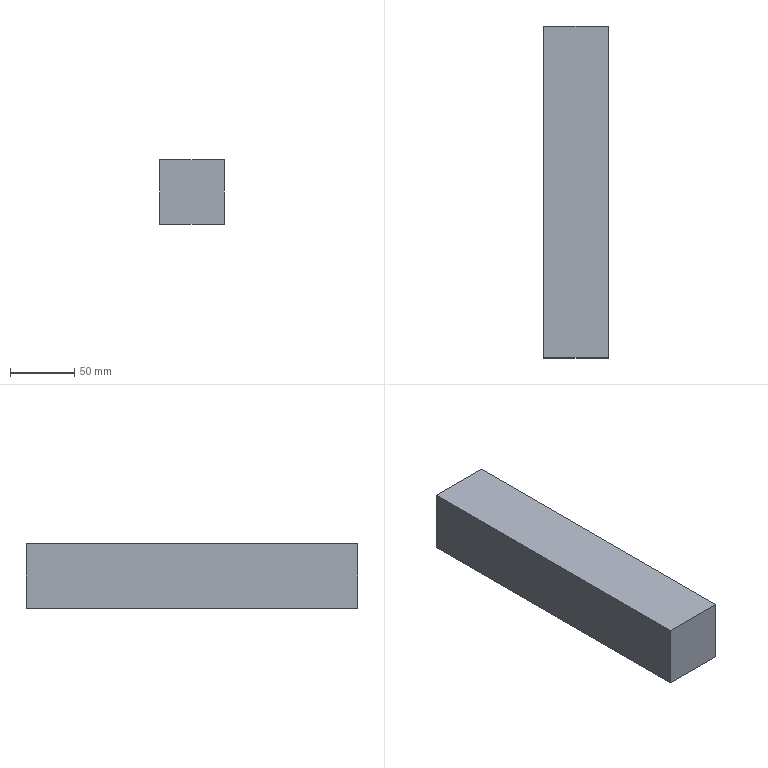Part | STEP file | 1 solid | 6 faces | box 50 x 259.164 x 50 mm | volume 647910 mm3 | plane 6
STEP:
#1=CARTESIAN_POINT('',(0.,0.,0.));
#2=DIRECTION('',(0.,0.,1.));
#3=DIRECTION('',(1.,0.,0.));
#4=AXIS2_PLACEMENT_3D('',#1,#2,#3);
#5=CARTESIAN_POINT('',(294.689,-240.836,393.641));
#6=VERTEX_POINT('',#5);
#7=CARTESIAN_POINT('',(294.689,-500.,393.641));
#8=VERTEX_POINT('',#7);
#9=CARTESIAN_POINT('',(294.689,-240.836,393.641));
#10=DIRECTION('',(0.,-1.,0.));
#11=VECTOR('',#10,1.);
#12=LINE('',#9,#11);
#13=CARTESIAN_POINT('',(294.689,-240.836,343.641));
#14=DIRECTION('',(1.,0.,0.));
#15=DIRECTION('',(0.,0.,1.));
#16=AXIS2_PLACEMENT_3D('',#13,#14,#15);
#17=PLANE('',#16);
#18=CARTESIAN_POINT('',(50.,0.));
#19=DIRECTION('',(0.,1.));
#20=VECTOR('',#19,1.);
#21=LINE('',#18,#20);
#22=(GEOMETRIC_REPRESENTATION_CONTEXT(2)PARAMETRIC_REPRESENTATION_CONTEXT()REPRESENTATION_CONTEXT('',''));
#23=DEFINITIONAL_REPRESENTATION('',(#21),#22);
#24=PCURVE('',#17,#23);
#25=CARTESIAN_POINT('',(0.,0.,393.641));
#26=DIRECTION('',(0.,0.,1.));
#27=DIRECTION('',(-1.,0.,0.));
#28=AXIS2_PLACEMENT_3D('',#25,#26,#27);
#29=PLANE('',#28);
#30=CARTESIAN_POINT('',(-294.689,240.836));
#31=DIRECTION('',(0.,1.));
#32=VECTOR('',#31,1.);
#33=LINE('',#30,#32);
#34=(GEOMETRIC_REPRESENTATION_CONTEXT(2)PARAMETRIC_REPRESENTATION_CONTEXT()REPRESENTATION_CONTEXT('',''));
#35=DEFINITIONAL_REPRESENTATION('',(#33),#34);
#36=PCURVE('',#29,#35);
#37=SURFACE_CURVE('',#12,(#24,#36),.PCURVE_S1.);
#38=EDGE_CURVE('',#6,#8,#37,.T.);
#39=ORIENTED_EDGE('',*,*,#38,.T.);
#40=CARTESIAN_POINT('',(294.689,-500.,343.641));
#41=VERTEX_POINT('',#40);
#42=CARTESIAN_POINT('',(294.689,-500.,343.641));
#43=DIRECTION('',(0.,0.,1.));
#44=VECTOR('',#43,1.);
#45=LINE('',#42,#44);
#46=CARTESIAN_POINT('',(0.,259.164));
#47=DIRECTION('',(1.,0.));
#48=VECTOR('',#47,1.);
#49=LINE('',#46,#48);
#50=(GEOMETRIC_REPRESENTATION_CONTEXT(2)PARAMETRIC_REPRESENTATION_CONTEXT()REPRESENTATION_CONTEXT('',''));
#51=DEFINITIONAL_REPRESENTATION('',(#49),#50);
#52=PCURVE('',#17,#51);
#53=CARTESIAN_POINT('',(294.689,-500.,343.641));
#54=DIRECTION('',(0.,-1.,0.));
#55=DIRECTION('',(-1.,0.,0.));
#56=AXIS2_PLACEMENT_3D('',#53,#54,#55);
#57=PLANE('',#56);
#58=CARTESIAN_POINT('',(0.,0.));
#59=DIRECTION('',(0.,-1.));
#60=VECTOR('',#59,1.);
#61=LINE('',#58,#60);
#62=(GEOMETRIC_REPRESENTATION_CONTEXT(2)PARAMETRIC_REPRESENTATION_CONTEXT()REPRESENTATION_CONTEXT('',''));
#63=DEFINITIONAL_REPRESENTATION('',(#61),#62);
#64=PCURVE('',#57,#63);
#65=SURFACE_CURVE('',#45,(#52,#64),.PCURVE_S1.);
#66=EDGE_CURVE('',#41,#8,#65,.T.);
#67=ORIENTED_EDGE('',*,*,#66,.F.);
#68=CARTESIAN_POINT('',(294.689,-240.836,343.641));
#69=VERTEX_POINT('',#68);
#70=CARTESIAN_POINT('',(294.689,-240.836,343.641));
#71=DIRECTION('',(0.,-1.,0.));
#72=VECTOR('',#71,1.);
#73=LINE('',#70,#72);
#74=CARTESIAN_POINT('',(0.,0.));
#75=DIRECTION('',(0.,1.));
#76=VECTOR('',#75,1.);
#77=LINE('',#74,#76);
#78=(GEOMETRIC_REPRESENTATION_CONTEXT(2)PARAMETRIC_REPRESENTATION_CONTEXT()REPRESENTATION_CONTEXT('',''));
#79=DEFINITIONAL_REPRESENTATION('',(#77),#78);
#80=PCURVE('',#17,#79);
#81=CARTESIAN_POINT('',(0.,0.,343.641));
#82=DIRECTION('',(0.,0.,1.));
#83=DIRECTION('',(-1.,0.,0.));
#84=AXIS2_PLACEMENT_3D('',#81,#82,#83);
#85=PLANE('',#84);
#86=CARTESIAN_POINT('',(-294.689,240.836));
#87=DIRECTION('',(0.,1.));
#88=VECTOR('',#87,1.);
#89=LINE('',#86,#88);
#90=(GEOMETRIC_REPRESENTATION_CONTEXT(2)PARAMETRIC_REPRESENTATION_CONTEXT()REPRESENTATION_CONTEXT('',''));
#91=DEFINITIONAL_REPRESENTATION('',(#89),#90);
#92=PCURVE('',#85,#91);
#93=SURFACE_CURVE('',#73,(#80,#92),.PCURVE_S1.);
#94=EDGE_CURVE('',#69,#41,#93,.T.);
#95=ORIENTED_EDGE('',*,*,#94,.F.);
#96=CARTESIAN_POINT('',(294.689,-240.836,343.641));
#97=DIRECTION('',(0.,0.,1.));
#98=VECTOR('',#97,1.);
#99=LINE('',#96,#98);
#100=CARTESIAN_POINT('',(0.,0.));
#101=DIRECTION('',(1.,0.));
#102=VECTOR('',#101,1.);
#103=LINE('',#100,#102);
#104=(GEOMETRIC_REPRESENTATION_CONTEXT(2)PARAMETRIC_REPRESENTATION_CONTEXT()REPRESENTATION_CONTEXT('',''));
#105=DEFINITIONAL_REPRESENTATION('',(#103),#104);
#106=PCURVE('',#17,#105);
#107=CARTESIAN_POINT('',(294.689,-240.836,343.641));
#108=DIRECTION('',(0.,1.,0.));
#109=DIRECTION('',(1.,0.,0.));
#110=AXIS2_PLACEMENT_3D('',#107,#108,#109);
#111=PLANE('',#110);
#112=CARTESIAN_POINT('',(0.,0.));
#113=DIRECTION('',(0.,-1.));
#114=VECTOR('',#113,1.);
#115=LINE('',#112,#114);
#116=(GEOMETRIC_REPRESENTATION_CONTEXT(2)PARAMETRIC_REPRESENTATION_CONTEXT()REPRESENTATION_CONTEXT('',''));
#117=DEFINITIONAL_REPRESENTATION('',(#115),#116);
#118=PCURVE('',#111,#117);
#119=SURFACE_CURVE('',#99,(#106,#118),.PCURVE_S1.);
#120=EDGE_CURVE('',#69,#6,#119,.T.);
#121=ORIENTED_EDGE('',*,*,#120,.T.);
#122=EDGE_LOOP('',(#39,#67,#95,#121));
#123=FACE_BOUND('',#122,.T.);
#124=ADVANCED_FACE('',(#123),#17,.T.);
#125=CARTESIAN_POINT('',(244.689,-240.836,393.641));
#126=VERTEX_POINT('',#125);
#127=CARTESIAN_POINT('',(294.689,-240.836,393.641));
#128=DIRECTION('',(1.,0.,0.));
#129=VECTOR('',#128,1.);
#130=LINE('',#127,#129);
#131=CARTESIAN_POINT('',(0.,-50.));
#132=DIRECTION('',(1.,0.));
#133=VECTOR('',#132,1.);
#134=LINE('',#131,#133);
#135=(GEOMETRIC_REPRESENTATION_CONTEXT(2)PARAMETRIC_REPRESENTATION_CONTEXT()REPRESENTATION_CONTEXT('',''));
#136=DEFINITIONAL_REPRESENTATION('',(#134),#135);
#137=PCURVE('',#111,#136);
#138=CARTESIAN_POINT('',(-294.689,240.836));
#139=DIRECTION('',(-1.,0.));
#140=VECTOR('',#139,1.);
#141=LINE('',#138,#140);
#142=(GEOMETRIC_REPRESENTATION_CONTEXT(2)PARAMETRIC_REPRESENTATION_CONTEXT()REPRESENTATION_CONTEXT('',''));
#143=DEFINITIONAL_REPRESENTATION('',(#141),#142);
#144=PCURVE('',#29,#143);
#145=SURFACE_CURVE('',#130,(#137,#144),.PCURVE_S1.);
#146=EDGE_CURVE('',#126,#6,#145,.T.);
#147=ORIENTED_EDGE('',*,*,#146,.T.);
#148=ORIENTED_EDGE('',*,*,#120,.F.);
#149=CARTESIAN_POINT('',(244.689,-240.836,343.641));
#150=VERTEX_POINT('',#149);
#151=CARTESIAN_POINT('',(294.689,-240.836,343.641));
#152=DIRECTION('',(1.,0.,0.));
#153=VECTOR('',#152,1.);
#154=LINE('',#151,#153);
#155=CARTESIAN_POINT('',(0.,0.));
#156=DIRECTION('',(1.,0.));
#157=VECTOR('',#156,1.);
#158=LINE('',#155,#157);
#159=(GEOMETRIC_REPRESENTATION_CONTEXT(2)PARAMETRIC_REPRESENTATION_CONTEXT()REPRESENTATION_CONTEXT('',''));
#160=DEFINITIONAL_REPRESENTATION('',(#158),#159);
#161=PCURVE('',#111,#160);
#162=CARTESIAN_POINT('',(-294.689,240.836));
#163=DIRECTION('',(-1.,0.));
#164=VECTOR('',#163,1.);
#165=LINE('',#162,#164);
#166=(GEOMETRIC_REPRESENTATION_CONTEXT(2)PARAMETRIC_REPRESENTATION_CONTEXT()REPRESENTATION_CONTEXT('',''));
#167=DEFINITIONAL_REPRESENTATION('',(#165),#166);
#168=PCURVE('',#85,#167);
#169=SURFACE_CURVE('',#154,(#161,#168),.PCURVE_S1.);
#170=EDGE_CURVE('',#150,#69,#169,.T.);
#171=ORIENTED_EDGE('',*,*,#170,.F.);
#172=CARTESIAN_POINT('',(244.689,-240.836,343.641));
#173=DIRECTION('',(0.,0.,1.));
#174=VECTOR('',#173,1.);
#175=LINE('',#172,#174);
#176=CARTESIAN_POINT('',(-50.,0.));
#177=DIRECTION('',(0.,-1.));
#178=VECTOR('',#177,1.);
#179=LINE('',#176,#178);
#180=(GEOMETRIC_REPRESENTATION_CONTEXT(2)PARAMETRIC_REPRESENTATION_CONTEXT()REPRESENTATION_CONTEXT('',''));
#181=DEFINITIONAL_REPRESENTATION('',(#179),#180);
#182=PCURVE('',#111,#181);
#183=CARTESIAN_POINT('',(244.689,-240.836,343.641));
#184=DIRECTION('',(-1.,0.,0.));
#185=DIRECTION('',(0.,1.,0.));
#186=AXIS2_PLACEMENT_3D('',#183,#184,#185);
#187=PLANE('',#186);
#188=CARTESIAN_POINT('',(0.,0.));
#189=DIRECTION('',(0.,-1.));
#190=VECTOR('',#189,1.);
#191=LINE('',#188,#190);
#192=(GEOMETRIC_REPRESENTATION_CONTEXT(2)PARAMETRIC_REPRESENTATION_CONTEXT()REPRESENTATION_CONTEXT('',''));
#193=DEFINITIONAL_REPRESENTATION('',(#191),#192);
#194=PCURVE('',#187,#193);
#195=SURFACE_CURVE('',#175,(#182,#194),.PCURVE_S1.);
#196=EDGE_CURVE('',#150,#126,#195,.T.);
#197=ORIENTED_EDGE('',*,*,#196,.T.);
#198=EDGE_LOOP('',(#147,#148,#171,#197));
#199=FACE_BOUND('',#198,.T.);
#200=ADVANCED_FACE('',(#199),#111,.T.);
#201=CARTESIAN_POINT('',(244.689,-500.,393.641));
#202=VERTEX_POINT('',#201);
#203=CARTESIAN_POINT('',(244.689,-240.836,393.641));
#204=DIRECTION('',(0.,1.,0.));
#205=VECTOR('',#204,1.);
#206=LINE('',#203,#205);
#207=CARTESIAN_POINT('',(0.,-50.));
#208=DIRECTION('',(1.,0.));
#209=VECTOR('',#208,1.);
#210=LINE('',#207,#209);
#211=(GEOMETRIC_REPRESENTATION_CONTEXT(2)PARAMETRIC_REPRESENTATION_CONTEXT()REPRESENTATION_CONTEXT('',''));
#212=DEFINITIONAL_REPRESENTATION('',(#210),#211);
#213=PCURVE('',#187,#212);
#214=CARTESIAN_POINT('',(-244.689,240.836));
#215=DIRECTION('',(0.,-1.));
#216=VECTOR('',#215,1.);
#217=LINE('',#214,#216);
#218=(GEOMETRIC_REPRESENTATION_CONTEXT(2)PARAMETRIC_REPRESENTATION_CONTEXT()REPRESENTATION_CONTEXT('',''));
#219=DEFINITIONAL_REPRESENTATION('',(#217),#218);
#220=PCURVE('',#29,#219);
#221=SURFACE_CURVE('',#206,(#213,#220),.PCURVE_S1.);
#222=EDGE_CURVE('',#202,#126,#221,.T.);
#223=ORIENTED_EDGE('',*,*,#222,.T.);
#224=ORIENTED_EDGE('',*,*,#196,.F.);
#225=CARTESIAN_POINT('',(244.689,-500.,343.641));
#226=VERTEX_POINT('',#225);
#227=CARTESIAN_POINT('',(244.689,-240.836,343.641));
#228=DIRECTION('',(0.,1.,0.));
#229=VECTOR('',#228,1.);
#230=LINE('',#227,#229);
#231=CARTESIAN_POINT('',(0.,0.));
#232=DIRECTION('',(1.,0.));
#233=VECTOR('',#232,1.);
#234=LINE('',#231,#233);
#235=(GEOMETRIC_REPRESENTATION_CONTEXT(2)PARAMETRIC_REPRESENTATION_CONTEXT()REPRESENTATION_CONTEXT('',''));
#236=DEFINITIONAL_REPRESENTATION('',(#234),#235);
#237=PCURVE('',#187,#236);
#238=CARTESIAN_POINT('',(-244.689,240.836));
#239=DIRECTION('',(0.,-1.));
#240=VECTOR('',#239,1.);
#241=LINE('',#238,#240);
#242=(GEOMETRIC_REPRESENTATION_CONTEXT(2)PARAMETRIC_REPRESENTATION_CONTEXT()REPRESENTATION_CONTEXT('',''));
#243=DEFINITIONAL_REPRESENTATION('',(#241),#242);
#244=PCURVE('',#85,#243);
#245=SURFACE_CURVE('',#230,(#237,#244),.PCURVE_S1.);
#246=EDGE_CURVE('',#226,#150,#245,.T.);
#247=ORIENTED_EDGE('',*,*,#246,.F.);
#248=CARTESIAN_POINT('',(244.689,-500.,343.641));
#249=DIRECTION('',(0.,0.,1.));
#250=VECTOR('',#249,1.);
#251=LINE('',#248,#250);
#252=CARTESIAN_POINT('',(-259.164,0.));
#253=DIRECTION('',(0.,-1.));
#254=VECTOR('',#253,1.);
#255=LINE('',#252,#254);
#256=(GEOMETRIC_REPRESENTATION_CONTEXT(2)PARAMETRIC_REPRESENTATION_CONTEXT()REPRESENTATION_CONTEXT('',''));
#257=DEFINITIONAL_REPRESENTATION('',(#255),#256);
#258=PCURVE('',#187,#257);
#259=CARTESIAN_POINT('',(50.,0.));
#260=DIRECTION('',(0.,-1.));
#261=VECTOR('',#260,1.);
#262=LINE('',#259,#261);
#263=(GEOMETRIC_REPRESENTATION_CONTEXT(2)PARAMETRIC_REPRESENTATION_CONTEXT()REPRESENTATION_CONTEXT('',''));
#264=DEFINITIONAL_REPRESENTATION('',(#262),#263);
#265=PCURVE('',#57,#264);
#266=SURFACE_CURVE('',#251,(#258,#265),.PCURVE_S1.);
#267=EDGE_CURVE('',#226,#202,#266,.T.);
#268=ORIENTED_EDGE('',*,*,#267,.T.);
#269=EDGE_LOOP('',(#223,#224,#247,#268));
#270=FACE_BOUND('',#269,.T.);
#271=ADVANCED_FACE('',(#270),#187,.T.);
#272=CARTESIAN_POINT('',(294.689,-500.,393.641));
#273=DIRECTION('',(-1.,0.,0.));
#274=VECTOR('',#273,1.);
#275=LINE('',#272,#274);
#276=CARTESIAN_POINT('',(0.,-50.));
#277=DIRECTION('',(1.,0.));
#278=VECTOR('',#277,1.);
#279=LINE('',#276,#278);
#280=(GEOMETRIC_REPRESENTATION_CONTEXT(2)PARAMETRIC_REPRESENTATION_CONTEXT()REPRESENTATION_CONTEXT('',''));
#281=DEFINITIONAL_REPRESENTATION('',(#279),#280);
#282=PCURVE('',#57,#281);
#283=CARTESIAN_POINT('',(-294.689,500.));
#284=DIRECTION('',(1.,0.));
#285=VECTOR('',#284,1.);
#286=LINE('',#283,#285);
#287=(GEOMETRIC_REPRESENTATION_CONTEXT(2)PARAMETRIC_REPRESENTATION_CONTEXT()REPRESENTATION_CONTEXT('',''));
#288=DEFINITIONAL_REPRESENTATION('',(#286),#287);
#289=PCURVE('',#29,#288);
#290=SURFACE_CURVE('',#275,(#282,#289),.PCURVE_S1.);
#291=EDGE_CURVE('',#8,#202,#290,.T.);
#292=ORIENTED_EDGE('',*,*,#291,.T.);
#293=ORIENTED_EDGE('',*,*,#267,.F.);
#294=CARTESIAN_POINT('',(294.689,-500.,343.641));
#295=DIRECTION('',(-1.,0.,0.));
#296=VECTOR('',#295,1.);
#297=LINE('',#294,#296);
#298=CARTESIAN_POINT('',(0.,0.));
#299=DIRECTION('',(1.,0.));
#300=VECTOR('',#299,1.);
#301=LINE('',#298,#300);
#302=(GEOMETRIC_REPRESENTATION_CONTEXT(2)PARAMETRIC_REPRESENTATION_CONTEXT()REPRESENTATION_CONTEXT('',''));
#303=DEFINITIONAL_REPRESENTATION('',(#301),#302);
#304=PCURVE('',#57,#303);
#305=CARTESIAN_POINT('',(-294.689,500.));
#306=DIRECTION('',(1.,0.));
#307=VECTOR('',#306,1.);
#308=LINE('',#305,#307);
#309=(GEOMETRIC_REPRESENTATION_CONTEXT(2)PARAMETRIC_REPRESENTATION_CONTEXT()REPRESENTATION_CONTEXT('',''));
#310=DEFINITIONAL_REPRESENTATION('',(#308),#309);
#311=PCURVE('',#85,#310);
#312=SURFACE_CURVE('',#297,(#304,#311),.PCURVE_S1.);
#313=EDGE_CURVE('',#41,#226,#312,.T.);
#314=ORIENTED_EDGE('',*,*,#313,.F.);
#315=ORIENTED_EDGE('',*,*,#66,.T.);
#316=EDGE_LOOP('',(#292,#293,#314,#315));
#317=FACE_BOUND('',#316,.T.);
#318=ADVANCED_FACE('',(#317),#57,.T.);
#319=ORIENTED_EDGE('',*,*,#94,.T.);
#320=ORIENTED_EDGE('',*,*,#313,.T.);
#321=ORIENTED_EDGE('',*,*,#246,.T.);
#322=ORIENTED_EDGE('',*,*,#170,.T.);
#323=EDGE_LOOP('',(#319,#320,#321,#322));
#324=FACE_BOUND('',#323,.T.);
#325=ADVANCED_FACE('',(#324),#85,.F.);
#326=ORIENTED_EDGE('',*,*,#38,.F.);
#327=ORIENTED_EDGE('',*,*,#146,.F.);
#328=ORIENTED_EDGE('',*,*,#222,.F.);
#329=ORIENTED_EDGE('',*,*,#291,.F.);
#330=EDGE_LOOP('',(#326,#327,#328,#329));
#331=FACE_BOUND('',#330,.T.);
#332=ADVANCED_FACE('',(#331),#29,.T.);
#333=CLOSED_SHELL('',(#124,#200,#271,#318,#325,#332));
#334=MANIFOLD_SOLID_BREP('',#333);
#335=(LENGTH_UNIT()NAMED_UNIT(*)SI_UNIT(.MILLI.,.METRE.));
#336=UNCERTAINTY_MEASURE_WITH_UNIT(LENGTH_MEASURE(0.0000001),#335,'','');
#337=(NAMED_UNIT(*)PLANE_ANGLE_UNIT()SI_UNIT($,.RADIAN.));
#338=(NAMED_UNIT(*)SI_UNIT($,.STERADIAN.)SOLID_ANGLE_UNIT());
#339=(GEOMETRIC_REPRESENTATION_CONTEXT(3)GLOBAL_UNCERTAINTY_ASSIGNED_CONTEXT((#336))GLOBAL_UNIT_ASSIGNED_CONTEXT((#335,#337,#338))REPRESENTATION_CONTEXT('',''));
#340=ADVANCED_BREP_SHAPE_REPRESENTATION('',(#4,#334),#339);